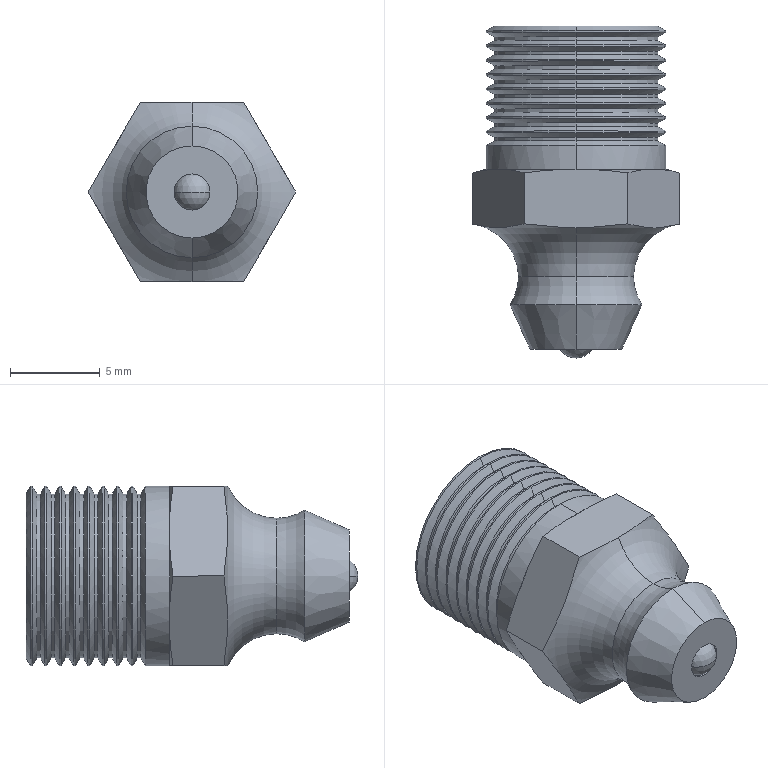Part | STEP file | KALAMITKA_1V11 | 2 solids | 115 faces | box 11.547 x 18.49 x 10 mm | volume 633.492 mm3 | cone 48 | cylinder 42 | plane 15 | torus 8 | sphere 2 | commonest cylinder face diameters 10 x18 9.134 x16 6.63 x4 2.007 x2 4.63 x2